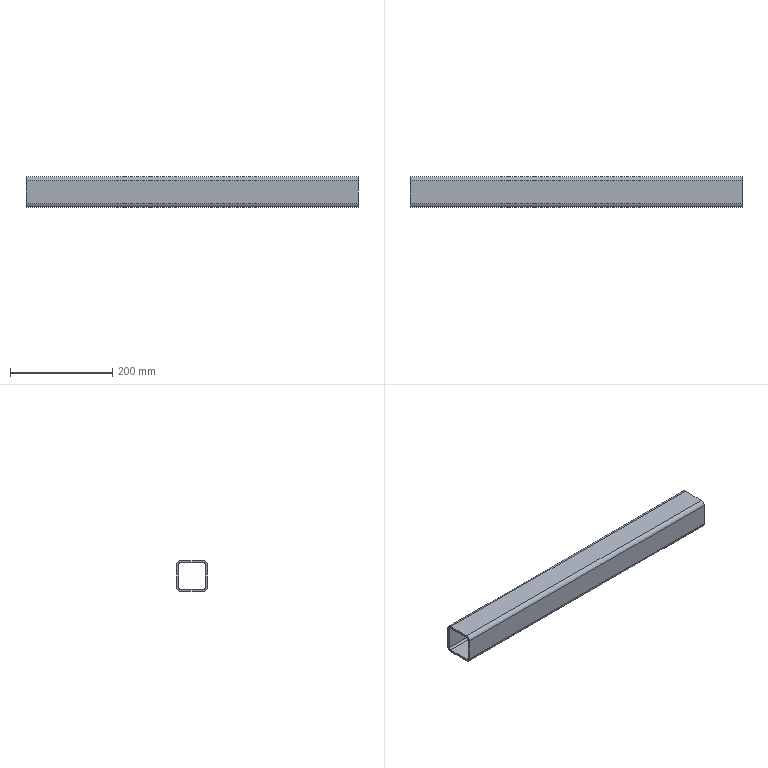Part | SolidWorks | features BaseBody 1 | 1 solid | 18 faces | box 650 x 60 x 60 mm | volume 555618 mm3 | plane 10 | cylinder 8 | commonest cylinder face diameters 8 x4 16 x4
STEP:
#1=CARTESIAN_POINT('',(-325.,1947.544,-76.));
#2=VERTEX_POINT('',#1);
#3=CARTESIAN_POINT('',(325.,1947.544,-76.));
#4=VERTEX_POINT('',#3);
#5=CARTESIAN_POINT('',(-325.,1947.544,-76.));
#6=DIRECTION('',(1.,0.,0.));
#7=VECTOR('',#6,1000.);
#8=LINE('',#5,#7);
#9=EDGE_CURVE('',#2,#4,#8,.T.);
#10=ORIENTED_EDGE('',*,*,#9,.T.);
#11=CARTESIAN_POINT('',(325.,1991.544,-76.));
#12=VERTEX_POINT('',#11);
#13=CARTESIAN_POINT('',(325.,1991.544,-76.));
#14=DIRECTION('',(0.,1.,0.));
#15=VECTOR('',#14,1000.);
#16=LINE('',#13,#15);
#17=EDGE_CURVE('',#4,#12,#16,.T.);
#18=ORIENTED_EDGE('',*,*,#17,.T.);
#19=CARTESIAN_POINT('',(-325.,1991.544,-76.));
#20=VERTEX_POINT('',#19);
#21=CARTESIAN_POINT('',(-325.,1991.544,-76.));
#22=DIRECTION('',(-1.,0.,0.));
#23=VECTOR('',#22,1000.);
#24=LINE('',#21,#23);
#25=EDGE_CURVE('',#12,#20,#24,.T.);
#26=ORIENTED_EDGE('',*,*,#25,.T.);
#27=CARTESIAN_POINT('',(-325.,1991.544,-76.));
#28=DIRECTION('',(0.,-1.,0.));
#29=VECTOR('',#28,1000.);
#30=LINE('',#27,#29);
#31=EDGE_CURVE('',#20,#2,#30,.T.);
#32=ORIENTED_EDGE('',*,*,#31,.T.);
#33=EDGE_LOOP('',(#10,#18,#26,#32));
#34=FACE_OUTER_BOUND('',#33,.T.);
#35=CARTESIAN_POINT('',(-325.,1991.544,-76.));
#36=DIRECTION('',(0.,0.,1.));
#37=DIRECTION('',(1.,0.,0.));
#38=AXIS2_PLACEMENT_3D('',#35,#36,#37);
#39=PLANE('',#38);
#40=ADVANCED_FACE('',(#34),#39,.T.);
#41=CARTESIAN_POINT('',(325.,1995.544,-72.));
#42=VERTEX_POINT('',#41);
#43=CARTESIAN_POINT('',(325.,1991.544,-72.));
#44=DIRECTION('',(1.,0.,0.));
#45=DIRECTION('',(0.,0.,-1.));
#46=AXIS2_PLACEMENT_3D('',#43,#44,#45);
#47=CIRCLE('',#46,4.);
#48=EDGE_CURVE('',#12,#42,#47,.T.);
#49=ORIENTED_EDGE('',*,*,#48,.F.);
#50=ORIENTED_EDGE('',*,*,#17,.F.);
#51=CARTESIAN_POINT('',(325.,1943.544,-72.));
#52=VERTEX_POINT('',#51);
#53=CARTESIAN_POINT('',(325.,1947.544,-72.));
#54=DIRECTION('',(1.,0.,0.));
#55=DIRECTION('',(0.,0.,-1.));
#56=AXIS2_PLACEMENT_3D('',#53,#54,#55);
#57=CIRCLE('',#56,4.);
#58=EDGE_CURVE('',#52,#4,#57,.T.);
#59=ORIENTED_EDGE('',*,*,#58,.F.);
#60=CARTESIAN_POINT('',(325.,1943.544,-28.));
#61=VERTEX_POINT('',#60);
#62=CARTESIAN_POINT('',(325.,1943.544,-28.));
#63=DIRECTION('',(0.,0.,-1.));
#64=VECTOR('',#63,1000.);
#65=LINE('',#62,#64);
#66=EDGE_CURVE('',#61,#52,#65,.T.);
#67=ORIENTED_EDGE('',*,*,#66,.F.);
#68=CARTESIAN_POINT('',(325.,1947.544,-24.));
#69=VERTEX_POINT('',#68);
#70=CARTESIAN_POINT('',(325.,1947.544,-28.));
#71=DIRECTION('',(1.,0.,0.));
#72=DIRECTION('',(0.,0.,-1.));
#73=AXIS2_PLACEMENT_3D('',#70,#71,#72);
#74=CIRCLE('',#73,4.);
#75=EDGE_CURVE('',#69,#61,#74,.T.);
#76=ORIENTED_EDGE('',*,*,#75,.F.);
#77=CARTESIAN_POINT('',(325.,1991.544,-24.));
#78=VERTEX_POINT('',#77);
#79=CARTESIAN_POINT('',(325.,1947.544,-24.));
#80=DIRECTION('',(0.,-1.,0.));
#81=VECTOR('',#80,1000.);
#82=LINE('',#79,#81);
#83=EDGE_CURVE('',#78,#69,#82,.T.);
#84=ORIENTED_EDGE('',*,*,#83,.F.);
#85=CARTESIAN_POINT('',(325.,1995.544,-28.));
#86=VERTEX_POINT('',#85);
#87=CARTESIAN_POINT('',(325.,1991.544,-28.));
#88=DIRECTION('',(1.,0.,0.));
#89=DIRECTION('',(0.,0.,-1.));
#90=AXIS2_PLACEMENT_3D('',#87,#88,#89);
#91=CIRCLE('',#90,4.);
#92=EDGE_CURVE('',#86,#78,#91,.T.);
#93=ORIENTED_EDGE('',*,*,#92,.F.);
#94=CARTESIAN_POINT('',(325.,1995.544,-28.));
#95=DIRECTION('',(0.,0.,1.));
#96=VECTOR('',#95,1000.);
#97=LINE('',#94,#96);
#98=EDGE_CURVE('',#42,#86,#97,.T.);
#99=ORIENTED_EDGE('',*,*,#98,.F.);
#100=EDGE_LOOP('',(#49,#50,#59,#67,#76,#84,#93,#99));
#101=FACE_BOUND('',#100,.T.);
#102=CARTESIAN_POINT('',(325.,1947.544,-80.));
#103=VERTEX_POINT('',#102);
#104=CARTESIAN_POINT('',(325.,1939.544,-72.));
#105=VERTEX_POINT('',#104);
#106=CARTESIAN_POINT('',(325.,1947.544,-72.));
#107=DIRECTION('',(-1.,0.,0.));
#108=DIRECTION('',(0.,0.,-1.));
#109=AXIS2_PLACEMENT_3D('',#106,#107,#108);
#110=CIRCLE('',#109,8.);
#111=EDGE_CURVE('',#103,#105,#110,.T.);
#112=ORIENTED_EDGE('',*,*,#111,.F.);
#113=CARTESIAN_POINT('',(325.,1991.544,-80.));
#114=VERTEX_POINT('',#113);
#115=CARTESIAN_POINT('',(325.,1947.544,-80.));
#116=DIRECTION('',(0.,-1.,0.));
#117=VECTOR('',#116,1000.);
#118=LINE('',#115,#117);
#119=EDGE_CURVE('',#114,#103,#118,.T.);
#120=ORIENTED_EDGE('',*,*,#119,.F.);
#121=CARTESIAN_POINT('',(325.,1999.544,-72.));
#122=VERTEX_POINT('',#121);
#123=CARTESIAN_POINT('',(325.,1991.544,-72.));
#124=DIRECTION('',(-1.,0.,0.));
#125=DIRECTION('',(0.,0.,-1.));
#126=AXIS2_PLACEMENT_3D('',#123,#124,#125);
#127=CIRCLE('',#126,8.);
#128=EDGE_CURVE('',#122,#114,#127,.T.);
#129=ORIENTED_EDGE('',*,*,#128,.F.);
#130=CARTESIAN_POINT('',(325.,1999.544,-28.));
#131=VERTEX_POINT('',#130);
#132=CARTESIAN_POINT('',(325.,1999.544,-28.));
#133=DIRECTION('',(0.,0.,-1.));
#134=VECTOR('',#133,1000.);
#135=LINE('',#132,#134);
#136=EDGE_CURVE('',#131,#122,#135,.T.);
#137=ORIENTED_EDGE('',*,*,#136,.F.);
#138=CARTESIAN_POINT('',(325.,1991.544,-20.));
#139=VERTEX_POINT('',#138);
#140=CARTESIAN_POINT('',(325.,1991.544,-28.));
#141=DIRECTION('',(-1.,0.,0.));
#142=DIRECTION('',(0.,0.,-1.));
#143=AXIS2_PLACEMENT_3D('',#140,#141,#142);
#144=CIRCLE('',#143,8.);
#145=EDGE_CURVE('',#139,#131,#144,.T.);
#146=ORIENTED_EDGE('',*,*,#145,.F.);
#147=CARTESIAN_POINT('',(325.,1947.544,-20.));
#148=VERTEX_POINT('',#147);
#149=CARTESIAN_POINT('',(325.,1947.544,-20.));
#150=DIRECTION('',(0.,1.,0.));
#151=VECTOR('',#150,1000.);
#152=LINE('',#149,#151);
#153=EDGE_CURVE('',#148,#139,#152,.T.);
#154=ORIENTED_EDGE('',*,*,#153,.F.);
#155=CARTESIAN_POINT('',(325.,1939.544,-28.));
#156=VERTEX_POINT('',#155);
#157=CARTESIAN_POINT('',(325.,1947.544,-28.));
#158=DIRECTION('',(-1.,0.,0.));
#159=DIRECTION('',(0.,0.,-1.));
#160=AXIS2_PLACEMENT_3D('',#157,#158,#159);
#161=CIRCLE('',#160,8.);
#162=EDGE_CURVE('',#156,#148,#161,.T.);
#163=ORIENTED_EDGE('',*,*,#162,.F.);
#164=CARTESIAN_POINT('',(325.,1939.544,-28.));
#165=DIRECTION('',(0.,0.,1.));
#166=VECTOR('',#165,1000.);
#167=LINE('',#164,#166);
#168=EDGE_CURVE('',#105,#156,#167,.T.);
#169=ORIENTED_EDGE('',*,*,#168,.F.);
#170=EDGE_LOOP('',(#112,#120,#129,#137,#146,#154,#163,#169));
#171=FACE_OUTER_BOUND('',#170,.T.);
#172=CARTESIAN_POINT('',(325.,1947.544,-28.));
#173=DIRECTION('',(-1.,0.,0.));
#174=DIRECTION('',(0.,0.,1.));
#175=AXIS2_PLACEMENT_3D('',#172,#173,#174);
#176=PLANE('',#175);
#177=ADVANCED_FACE('',(#101,#171),#176,.F.);
#178=CARTESIAN_POINT('',(-325.,1943.544,-72.));
#179=VERTEX_POINT('',#178);
#180=CARTESIAN_POINT('',(-325.,1947.544,-72.));
#181=DIRECTION('',(1.,0.,0.));
#182=DIRECTION('',(0.,0.,-1.));
#183=AXIS2_PLACEMENT_3D('',#180,#181,#182);
#184=CIRCLE('',#183,4.);
#185=EDGE_CURVE('',#179,#2,#184,.T.);
#186=ORIENTED_EDGE('',*,*,#185,.F.);
#187=CARTESIAN_POINT('',(-325.,1943.544,-72.));
#188=DIRECTION('',(-1.,0.,0.));
#189=VECTOR('',#188,1000.);
#190=LINE('',#187,#189);
#191=EDGE_CURVE('',#52,#179,#190,.T.);
#192=ORIENTED_EDGE('',*,*,#191,.F.);
#193=ORIENTED_EDGE('',*,*,#58,.T.);
#194=ORIENTED_EDGE('',*,*,#9,.F.);
#195=EDGE_LOOP('',(#186,#192,#193,#194));
#196=FACE_OUTER_BOUND('',#195,.T.);
#197=CARTESIAN_POINT('',(-325.,1947.544,-72.));
#198=DIRECTION('',(1.,0.,0.));
#199=DIRECTION('',(0.,0.,-1.));
#200=AXIS2_PLACEMENT_3D('',#197,#198,#199);
#201=CYLINDRICAL_SURFACE('',#200,4.);
#202=ADVANCED_FACE('',(#196),#201,.F.);
#203=CARTESIAN_POINT('',(-325.,1995.544,-72.));
#204=VERTEX_POINT('',#203);
#205=CARTESIAN_POINT('',(-325.,1995.544,-28.));
#206=VERTEX_POINT('',#205);
#207=CARTESIAN_POINT('',(-325.,1995.544,-28.));
#208=DIRECTION('',(0.,0.,1.));
#209=VECTOR('',#208,1000.);
#210=LINE('',#207,#209);
#211=EDGE_CURVE('',#204,#206,#210,.T.);
#212=ORIENTED_EDGE('',*,*,#211,.T.);
#213=CARTESIAN_POINT('',(-325.,1991.544,-24.));
#214=VERTEX_POINT('',#213);
#215=CARTESIAN_POINT('',(-325.,1991.544,-28.));
#216=DIRECTION('',(1.,0.,0.));
#217=DIRECTION('',(0.,0.,-1.));
#218=AXIS2_PLACEMENT_3D('',#215,#216,#217);
#219=CIRCLE('',#218,4.);
#220=EDGE_CURVE('',#206,#214,#219,.T.);
#221=ORIENTED_EDGE('',*,*,#220,.T.);
#222=CARTESIAN_POINT('',(-325.,1947.544,-24.));
#223=VERTEX_POINT('',#222);
#224=CARTESIAN_POINT('',(-325.,1947.544,-24.));
#225=DIRECTION('',(0.,-1.,0.));
#226=VECTOR('',#225,1000.);
#227=LINE('',#224,#226);
#228=EDGE_CURVE('',#214,#223,#227,.T.);
#229=ORIENTED_EDGE('',*,*,#228,.T.);
#230=CARTESIAN_POINT('',(-325.,1943.544,-28.));
#231=VERTEX_POINT('',#230);
#232=CARTESIAN_POINT('',(-325.,1947.544,-28.));
#233=DIRECTION('',(1.,0.,0.));
#234=DIRECTION('',(0.,0.,-1.));
#235=AXIS2_PLACEMENT_3D('',#232,#233,#234);
#236=CIRCLE('',#235,4.);
#237=EDGE_CURVE('',#223,#231,#236,.T.);
#238=ORIENTED_EDGE('',*,*,#237,.T.);
#239=CARTESIAN_POINT('',(-325.,1943.544,-28.));
#240=DIRECTION('',(0.,0.,-1.));
#241=VECTOR('',#240,1000.);
#242=LINE('',#239,#241);
#243=EDGE_CURVE('',#231,#179,#242,.T.);
#244=ORIENTED_EDGE('',*,*,#243,.T.);
#245=ORIENTED_EDGE('',*,*,#185,.T.);
#246=ORIENTED_EDGE('',*,*,#31,.F.);
#247=CARTESIAN_POINT('',(-325.,1991.544,-72.));
#248=DIRECTION('',(1.,0.,0.));
#249=DIRECTION('',(0.,0.,-1.));
#250=AXIS2_PLACEMENT_3D('',#247,#248,#249);
#251=CIRCLE('',#250,4.);
#252=EDGE_CURVE('',#20,#204,#251,.T.);
#253=ORIENTED_EDGE('',*,*,#252,.T.);
#254=EDGE_LOOP('',(#212,#221,#229,#238,#244,#245,#246,#253));
#255=FACE_BOUND('',#254,.T.);
#256=CARTESIAN_POINT('',(-325.,1939.544,-72.));
#257=VERTEX_POINT('',#256);
#258=CARTESIAN_POINT('',(-325.,1939.544,-28.));
#259=VERTEX_POINT('',#258);
#260=CARTESIAN_POINT('',(-325.,1939.544,-28.));
#261=DIRECTION('',(0.,0.,1.));
#262=VECTOR('',#261,1000.);
#263=LINE('',#260,#262);
#264=EDGE_CURVE('',#257,#259,#263,.T.);
#265=ORIENTED_EDGE('',*,*,#264,.T.);
#266=CARTESIAN_POINT('',(-325.,1947.544,-20.));
#267=VERTEX_POINT('',#266);
#268=CARTESIAN_POINT('',(-325.,1947.544,-28.));
#269=DIRECTION('',(-1.,0.,0.));
#270=DIRECTION('',(0.,0.,-1.));
#271=AXIS2_PLACEMENT_3D('',#268,#269,#270);
#272=CIRCLE('',#271,8.);
#273=EDGE_CURVE('',#259,#267,#272,.T.);
#274=ORIENTED_EDGE('',*,*,#273,.T.);
#275=CARTESIAN_POINT('',(-325.,1991.544,-20.));
#276=VERTEX_POINT('',#275);
#277=CARTESIAN_POINT('',(-325.,1947.544,-20.));
#278=DIRECTION('',(0.,1.,0.));
#279=VECTOR('',#278,1000.);
#280=LINE('',#277,#279);
#281=EDGE_CURVE('',#267,#276,#280,.T.);
#282=ORIENTED_EDGE('',*,*,#281,.T.);
#283=CARTESIAN_POINT('',(-325.,1999.544,-28.));
#284=VERTEX_POINT('',#283);
#285=CARTESIAN_POINT('',(-325.,1991.544,-28.));
#286=DIRECTION('',(-1.,0.,0.));
#287=DIRECTION('',(0.,0.,-1.));
#288=AXIS2_PLACEMENT_3D('',#285,#286,#287);
#289=CIRCLE('',#288,8.);
#290=EDGE_CURVE('',#276,#284,#289,.T.);
#291=ORIENTED_EDGE('',*,*,#290,.T.);
#292=CARTESIAN_POINT('',(-325.,1999.544,-72.));
#293=VERTEX_POINT('',#292);
#294=CARTESIAN_POINT('',(-325.,1999.544,-28.));
#295=DIRECTION('',(0.,0.,-1.));
#296=VECTOR('',#295,1000.);
#297=LINE('',#294,#296);
#298=EDGE_CURVE('',#284,#293,#297,.T.);
#299=ORIENTED_EDGE('',*,*,#298,.T.);
#300=CARTESIAN_POINT('',(-325.,1991.544,-80.));
#301=VERTEX_POINT('',#300);
#302=CARTESIAN_POINT('',(-325.,1991.544,-72.));
#303=DIRECTION('',(-1.,0.,0.));
#304=DIRECTION('',(0.,0.,-1.));
#305=AXIS2_PLACEMENT_3D('',#302,#303,#304);
#306=CIRCLE('',#305,8.);
#307=EDGE_CURVE('',#293,#301,#306,.T.);
#308=ORIENTED_EDGE('',*,*,#307,.T.);
#309=CARTESIAN_POINT('',(-325.,1947.544,-80.));
#310=VERTEX_POINT('',#309);
#311=CARTESIAN_POINT('',(-325.,1947.544,-80.));
#312=DIRECTION('',(0.,-1.,0.));
#313=VECTOR('',#312,1000.);
#314=LINE('',#311,#313);
#315=EDGE_CURVE('',#301,#310,#314,.T.);
#316=ORIENTED_EDGE('',*,*,#315,.T.);
#317=CARTESIAN_POINT('',(-325.,1947.544,-72.));
#318=DIRECTION('',(-1.,0.,0.));
#319=DIRECTION('',(0.,0.,-1.));
#320=AXIS2_PLACEMENT_3D('',#317,#318,#319);
#321=CIRCLE('',#320,8.);
#322=EDGE_CURVE('',#310,#257,#321,.T.);
#323=ORIENTED_EDGE('',*,*,#322,.T.);
#324=EDGE_LOOP('',(#265,#274,#282,#291,#299,#308,#316,#323));
#325=FACE_OUTER_BOUND('',#324,.T.);
#326=CARTESIAN_POINT('',(-325.,1947.544,-28.));
#327=DIRECTION('',(-1.,0.,0.));
#328=DIRECTION('',(0.,0.,1.));
#329=AXIS2_PLACEMENT_3D('',#326,#327,#328);
#330=PLANE('',#329);
#331=ADVANCED_FACE('',(#255,#325),#330,.T.);
#332=ORIENTED_EDGE('',*,*,#252,.F.);
#333=ORIENTED_EDGE('',*,*,#25,.F.);
#334=ORIENTED_EDGE('',*,*,#48,.T.);
#335=CARTESIAN_POINT('',(-325.,1995.544,-72.));
#336=DIRECTION('',(1.,0.,0.));
#337=VECTOR('',#336,1000.);
#338=LINE('',#335,#337);
#339=EDGE_CURVE('',#204,#42,#338,.T.);
#340=ORIENTED_EDGE('',*,*,#339,.F.);
#341=EDGE_LOOP('',(#332,#333,#334,#340));
#342=FACE_OUTER_BOUND('',#341,.T.);
#343=CARTESIAN_POINT('',(-325.,1991.544,-72.));
#344=DIRECTION('',(1.,0.,0.));
#345=DIRECTION('',(0.,0.,-1.));
#346=AXIS2_PLACEMENT_3D('',#343,#344,#345);
#347=CYLINDRICAL_SURFACE('',#346,4.);
#348=ADVANCED_FACE('',(#342),#347,.F.);
#349=ORIENTED_EDGE('',*,*,#339,.T.);
#350=ORIENTED_EDGE('',*,*,#98,.T.);
#351=CARTESIAN_POINT('',(-325.,1995.544,-28.));
#352=DIRECTION('',(-1.,0.,0.));
#353=VECTOR('',#352,1000.);
#354=LINE('',#351,#353);
#355=EDGE_CURVE('',#86,#206,#354,.T.);
#356=ORIENTED_EDGE('',*,*,#355,.T.);
#357=ORIENTED_EDGE('',*,*,#211,.F.);
#358=EDGE_LOOP('',(#349,#350,#356,#357));
#359=FACE_OUTER_BOUND('',#358,.T.);
#360=CARTESIAN_POINT('',(-325.,1995.544,-72.));
#361=DIRECTION('',(0.,-1.,0.));
#362=DIRECTION('',(0.,0.,-1.));
#363=AXIS2_PLACEMENT_3D('',#360,#361,#362);
#364=PLANE('',#363);
#365=ADVANCED_FACE('',(#359),#364,.T.);
#366=CARTESIAN_POINT('',(-325.,1943.544,-28.));
#367=DIRECTION('',(1.,0.,0.));
#368=VECTOR('',#367,1000.);
#369=LINE('',#366,#368);
#370=EDGE_CURVE('',#231,#61,#369,.T.);
#371=ORIENTED_EDGE('',*,*,#370,.T.);
#372=ORIENTED_EDGE('',*,*,#66,.T.);
#373=ORIENTED_EDGE('',*,*,#191,.T.);
#374=ORIENTED_EDGE('',*,*,#243,.F.);
#375=EDGE_LOOP('',(#371,#372,#373,#374));
#376=FACE_OUTER_BOUND('',#375,.T.);
#377=CARTESIAN_POINT('',(-325.,1943.544,-28.));
#378=DIRECTION('',(0.,1.,0.));
#379=DIRECTION('',(0.,0.,1.));
#380=AXIS2_PLACEMENT_3D('',#377,#378,#379);
#381=PLANE('',#380);
#382=ADVANCED_FACE('',(#376),#381,.T.);
#383=ORIENTED_EDGE('',*,*,#237,.F.);
#384=CARTESIAN_POINT('',(-325.,1947.544,-24.));
#385=DIRECTION('',(-1.,0.,0.));
#386=VECTOR('',#385,1000.);
#387=LINE('',#384,#386);
#388=EDGE_CURVE('',#69,#223,#387,.T.);
#389=ORIENTED_EDGE('',*,*,#388,.F.);
#390=ORIENTED_EDGE('',*,*,#75,.T.);
#391=ORIENTED_EDGE('',*,*,#370,.F.);
#392=EDGE_LOOP('',(#383,#389,#390,#391));
#393=FACE_OUTER_BOUND('',#392,.T.);
#394=CARTESIAN_POINT('',(-325.,1947.544,-28.));
#395=DIRECTION('',(1.,0.,0.));
#396=DIRECTION('',(0.,0.,-1.));
#397=AXIS2_PLACEMENT_3D('',#394,#395,#396);
#398=CYLINDRICAL_SURFACE('',#397,4.);
#399=ADVANCED_FACE('',(#393),#398,.F.);
#400=CARTESIAN_POINT('',(-325.,1991.544,-24.));
#401=DIRECTION('',(1.,0.,0.));
#402=VECTOR('',#401,1000.);
#403=LINE('',#400,#402);
#404=EDGE_CURVE('',#214,#78,#403,.T.);
#405=ORIENTED_EDGE('',*,*,#404,.T.);
#406=ORIENTED_EDGE('',*,*,#83,.T.);
#407=ORIENTED_EDGE('',*,*,#388,.T.);
#408=ORIENTED_EDGE('',*,*,#228,.F.);
#409=EDGE_LOOP('',(#405,#406,#407,#408));
#410=FACE_OUTER_BOUND('',#409,.T.);
#411=CARTESIAN_POINT('',(-325.,1947.544,-24.));
#412=DIRECTION('',(0.,0.,-1.));
#413=DIRECTION('',(-1.,0.,0.));
#414=AXIS2_PLACEMENT_3D('',#411,#412,#413);
#415=PLANE('',#414);
#416=ADVANCED_FACE('',(#410),#415,.T.);
#417=ORIENTED_EDGE('',*,*,#220,.F.);
#418=ORIENTED_EDGE('',*,*,#355,.F.);
#419=ORIENTED_EDGE('',*,*,#92,.T.);
#420=ORIENTED_EDGE('',*,*,#404,.F.);
#421=EDGE_LOOP('',(#417,#418,#419,#420));
#422=FACE_OUTER_BOUND('',#421,.T.);
#423=CARTESIAN_POINT('',(-325.,1991.544,-28.));
#424=DIRECTION('',(1.,0.,0.));
#425=DIRECTION('',(0.,0.,-1.));
#426=AXIS2_PLACEMENT_3D('',#423,#424,#425);
#427=CYLINDRICAL_SURFACE('',#426,4.);
#428=ADVANCED_FACE('',(#422),#427,.F.);
#429=ORIENTED_EDGE('',*,*,#264,.F.);
#430=CARTESIAN_POINT('',(-325.,1939.544,-72.));
#431=DIRECTION('',(-1.,0.,0.));
#432=VECTOR('',#431,1000.);
#433=LINE('',#430,#432);
#434=EDGE_CURVE('',#105,#257,#433,.T.);
#435=ORIENTED_EDGE('',*,*,#434,.F.);
#436=ORIENTED_EDGE('',*,*,#168,.T.);
#437=CARTESIAN_POINT('',(-325.,1939.544,-28.));
#438=DIRECTION('',(1.,0.,0.));
#439=VECTOR('',#438,1000.);
#440=LINE('',#437,#439);
#441=EDGE_CURVE('',#259,#156,#440,.T.);
#442=ORIENTED_EDGE('',*,*,#441,.F.);
#443=EDGE_LOOP('',(#429,#435,#436,#442));
#444=FACE_OUTER_BOUND('',#443,.T.);
#445=CARTESIAN_POINT('',(-325.,1939.544,-28.));
#446=DIRECTION('',(0.,1.,0.));
#447=DIRECTION('',(0.,0.,1.));
#448=AXIS2_PLACEMENT_3D('',#445,#446,#447);
#449=PLANE('',#448);
#450=ADVANCED_FACE('',(#444),#449,.F.);
#451=CARTESIAN_POINT('',(-325.,1947.544,-80.));
#452=DIRECTION('',(1.,0.,0.));
#453=VECTOR('',#452,1000.);
#454=LINE('',#451,#453);
#455=EDGE_CURVE('',#310,#103,#454,.T.);
#456=ORIENTED_EDGE('',*,*,#455,.T.);
#457=ORIENTED_EDGE('',*,*,#111,.T.);
#458=ORIENTED_EDGE('',*,*,#434,.T.);
#459=ORIENTED_EDGE('',*,*,#322,.F.);
#460=EDGE_LOOP('',(#456,#457,#458,#459));
#461=FACE_OUTER_BOUND('',#460,.T.);
#462=CARTESIAN_POINT('',(-325.,1947.544,-72.));
#463=DIRECTION('',(1.,0.,0.));
#464=DIRECTION('',(0.,0.,-1.));
#465=AXIS2_PLACEMENT_3D('',#462,#463,#464);
#466=CYLINDRICAL_SURFACE('',#465,8.);
#467=ADVANCED_FACE('',(#461),#466,.T.);
#468=ORIENTED_EDGE('',*,*,#315,.F.);
#469=CARTESIAN_POINT('',(-325.,1991.544,-80.));
#470=DIRECTION('',(-1.,0.,0.));
#471=VECTOR('',#470,1000.);
#472=LINE('',#469,#471);
#473=EDGE_CURVE('',#114,#301,#472,.T.);
#474=ORIENTED_EDGE('',*,*,#473,.F.);
#475=ORIENTED_EDGE('',*,*,#119,.T.);
#476=ORIENTED_EDGE('',*,*,#455,.F.);
#477=EDGE_LOOP('',(#468,#474,#475,#476));
#478=FACE_OUTER_BOUND('',#477,.T.);
#479=CARTESIAN_POINT('',(-325.,1991.544,-80.));
#480=DIRECTION('',(0.,0.,1.));
#481=DIRECTION('',(1.,0.,0.));
#482=AXIS2_PLACEMENT_3D('',#479,#480,#481);
#483=PLANE('',#482);
#484=ADVANCED_FACE('',(#478),#483,.F.);
#485=CARTESIAN_POINT('',(-325.,1999.544,-72.));
#486=DIRECTION('',(1.,0.,0.));
#487=VECTOR('',#486,1000.);
#488=LINE('',#485,#487);
#489=EDGE_CURVE('',#293,#122,#488,.T.);
#490=ORIENTED_EDGE('',*,*,#489,.T.);
#491=ORIENTED_EDGE('',*,*,#128,.T.);
#492=ORIENTED_EDGE('',*,*,#473,.T.);
#493=ORIENTED_EDGE('',*,*,#307,.F.);
#494=EDGE_LOOP('',(#490,#491,#492,#493));
#495=FACE_OUTER_BOUND('',#494,.T.);
#496=CARTESIAN_POINT('',(-325.,1991.544,-72.));
#497=DIRECTION('',(1.,0.,0.));
#498=DIRECTION('',(0.,0.,-1.));
#499=AXIS2_PLACEMENT_3D('',#496,#497,#498);
#500=CYLINDRICAL_SURFACE('',#499,8.);
#501=ADVANCED_FACE('',(#495),#500,.T.);
#502=ORIENTED_EDGE('',*,*,#298,.F.);
#503=CARTESIAN_POINT('',(-325.,1999.544,-28.));
#504=DIRECTION('',(-1.,0.,0.));
#505=VECTOR('',#504,1000.);
#506=LINE('',#503,#505);
#507=EDGE_CURVE('',#131,#284,#506,.T.);
#508=ORIENTED_EDGE('',*,*,#507,.F.);
#509=ORIENTED_EDGE('',*,*,#136,.T.);
#510=ORIENTED_EDGE('',*,*,#489,.F.);
#511=EDGE_LOOP('',(#502,#508,#509,#510));
#512=FACE_OUTER_BOUND('',#511,.T.);
#513=CARTESIAN_POINT('',(-325.,1999.544,-72.));
#514=DIRECTION('',(0.,-1.,0.));
#515=DIRECTION('',(0.,0.,-1.));
#516=AXIS2_PLACEMENT_3D('',#513,#514,#515);
#517=PLANE('',#516);
#518=ADVANCED_FACE('',(#512),#517,.F.);
#519=CARTESIAN_POINT('',(-325.,1991.544,-20.));
#520=DIRECTION('',(1.,0.,0.));
#521=VECTOR('',#520,1000.);
#522=LINE('',#519,#521);
#523=EDGE_CURVE('',#276,#139,#522,.T.);
#524=ORIENTED_EDGE('',*,*,#523,.T.);
#525=ORIENTED_EDGE('',*,*,#145,.T.);
#526=ORIENTED_EDGE('',*,*,#507,.T.);
#527=ORIENTED_EDGE('',*,*,#290,.F.);
#528=EDGE_LOOP('',(#524,#525,#526,#527));
#529=FACE_OUTER_BOUND('',#528,.T.);
#530=CARTESIAN_POINT('',(-325.,1991.544,-28.));
#531=DIRECTION('',(1.,0.,0.));
#532=DIRECTION('',(0.,0.,-1.));
#533=AXIS2_PLACEMENT_3D('',#530,#531,#532);
#534=CYLINDRICAL_SURFACE('',#533,8.);
#535=ADVANCED_FACE('',(#529),#534,.T.);
#536=ORIENTED_EDGE('',*,*,#281,.F.);
#537=CARTESIAN_POINT('',(-325.,1947.544,-20.));
#538=DIRECTION('',(-1.,0.,0.));
#539=VECTOR('',#538,1000.);
#540=LINE('',#537,#539);
#541=EDGE_CURVE('',#148,#267,#540,.T.);
#542=ORIENTED_EDGE('',*,*,#541,.F.);
#543=ORIENTED_EDGE('',*,*,#153,.T.);
#544=ORIENTED_EDGE('',*,*,#523,.F.);
#545=EDGE_LOOP('',(#536,#542,#543,#544));
#546=FACE_OUTER_BOUND('',#545,.T.);
#547=CARTESIAN_POINT('',(-325.,1947.544,-20.));
#548=DIRECTION('',(0.,0.,-1.));
#549=DIRECTION('',(-1.,0.,0.));
#550=AXIS2_PLACEMENT_3D('',#547,#548,#549);
#551=PLANE('',#550);
#552=ADVANCED_FACE('',(#546),#551,.F.);
#553=ORIENTED_EDGE('',*,*,#441,.T.);
#554=ORIENTED_EDGE('',*,*,#162,.T.);
#555=ORIENTED_EDGE('',*,*,#541,.T.);
#556=ORIENTED_EDGE('',*,*,#273,.F.);
#557=EDGE_LOOP('',(#553,#554,#555,#556));
#558=FACE_OUTER_BOUND('',#557,.T.);
#559=CARTESIAN_POINT('',(-325.,1947.544,-28.));
#560=DIRECTION('',(1.,0.,0.));
#561=DIRECTION('',(0.,0.,-1.));
#562=AXIS2_PLACEMENT_3D('',#559,#560,#561);
#563=CYLINDRICAL_SURFACE('',#562,8.);
#564=ADVANCED_FACE('',(#558),#563,.T.);
#565=CLOSED_SHELL('',(#40,#177,#202,#331,#348,#365,#382,#399,#416,#428,#450,#467,#484,#501,#518,#535,#552,#564));
#566=MANIFOLD_SOLID_BREP('',#565);
#567=CARTESIAN_POINT('',(0.,0.,0.));
#568=DIRECTION('',(0.,0.,1.));
#569=DIRECTION('',(1.,0.,0.));
#570=AXIS2_PLACEMENT_3D('',#567,#568,#569);
#571=(LENGTH_UNIT()NAMED_UNIT(*)SI_UNIT(.MILLI.,.METRE.));
#572=UNCERTAINTY_MEASURE_WITH_UNIT(LENGTH_MEASURE(0.00001),#571,'','');
#573=(NAMED_UNIT(*)PLANE_ANGLE_UNIT()SI_UNIT($,.RADIAN.));
#574=(NAMED_UNIT(*)SI_UNIT($,.STERADIAN.)SOLID_ANGLE_UNIT());
#575=(GEOMETRIC_REPRESENTATION_CONTEXT(3)GLOBAL_UNCERTAINTY_ASSIGNED_CONTEXT((#572))GLOBAL_UNIT_ASSIGNED_CONTEXT((#571,#573,#574))REPRESENTATION_CONTEXT('',''));
#576=ADVANCED_BREP_SHAPE_REPRESENTATION('',(#566,#570),#575);